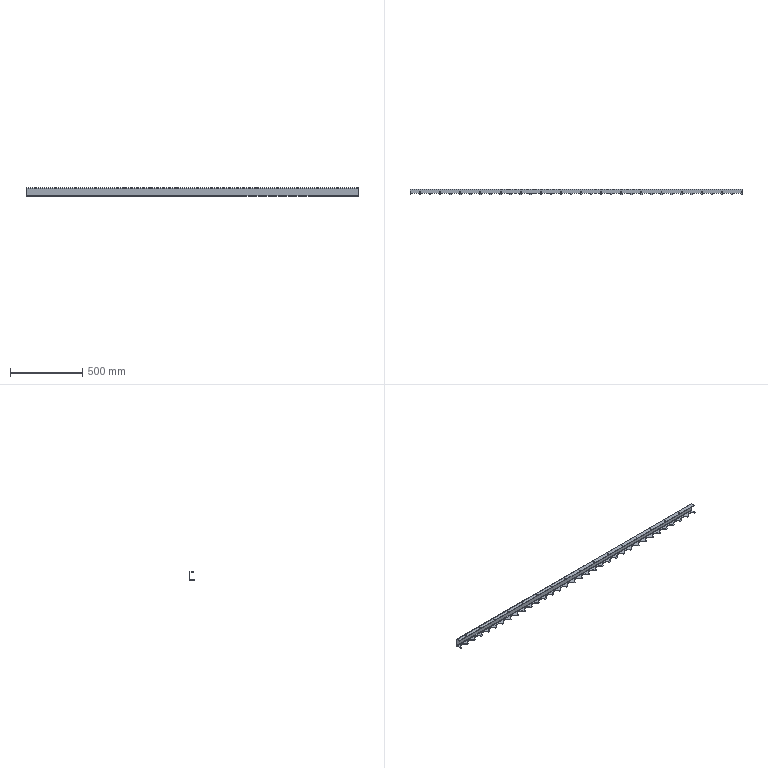Part | STEP file | cc-coverrollers-32 | 1 solid | 98 faces | box 2303 x 40 x 60 mm | volume 607914 mm3 | plane 44 | cylinder 37 | spline 17 | commonest cylinder face diameters 60 x33 5 x2 10 x2